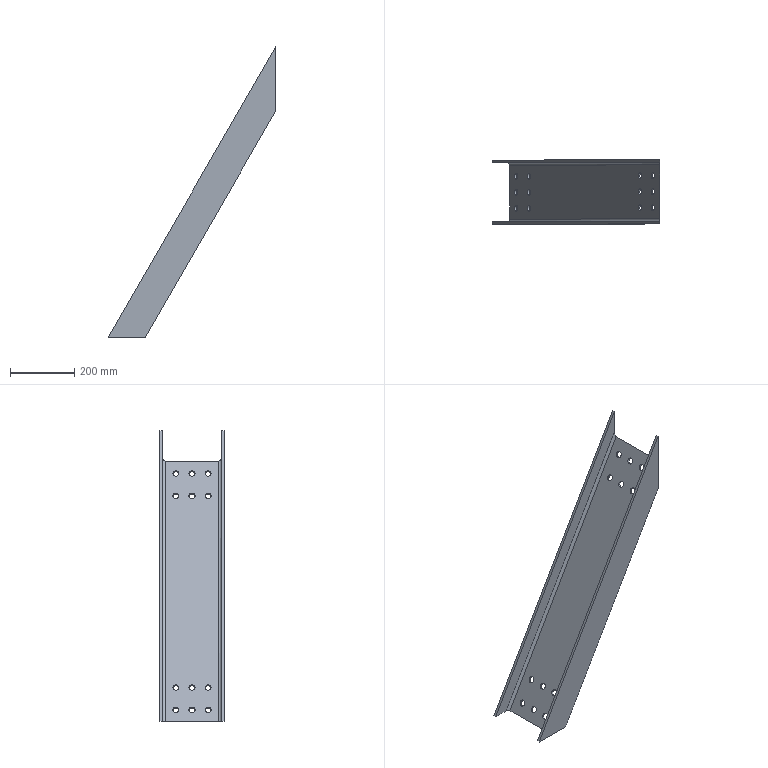Part | STEP file | 粉仓Diagonal Brace梁9_Default<As Machined> | 1 solid | 42 faces | box 522.735 x 200 x 905.404 mm | volume 2461540 mm3 | cylinder 28 | plane 14 | commonest cylinder face diameters 19 x24 16 x4